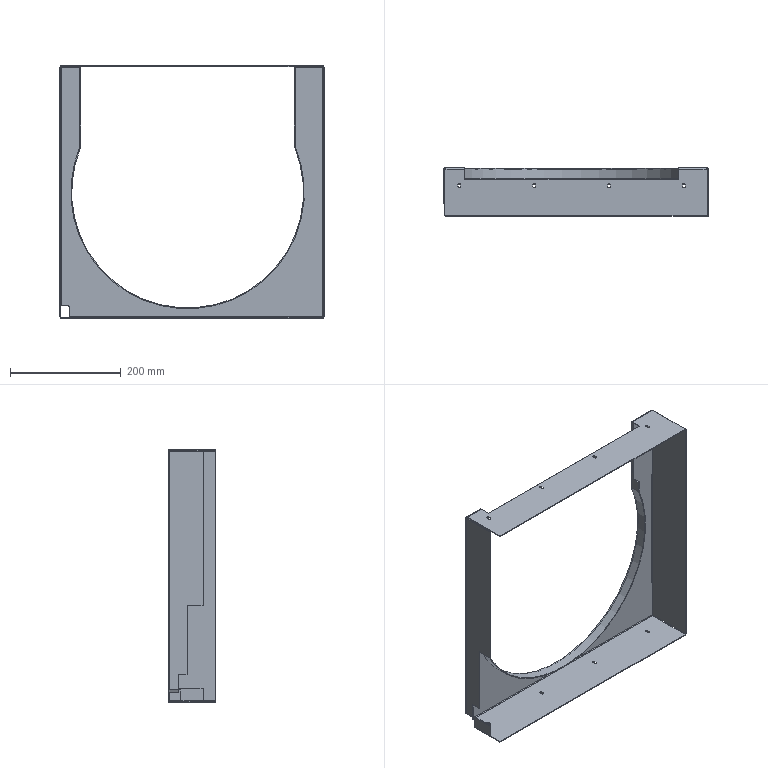Part | NX | features BREP 1 | 1 solid | 121 faces | box 477 x 86 x 455 mm | volume 309171 mm3 | plane 68 | cylinder 47 | spline 6 | commonest cylinder face diameters 4.5 x24 2 x15 5 x5 4 x1 418 x1 421 x1